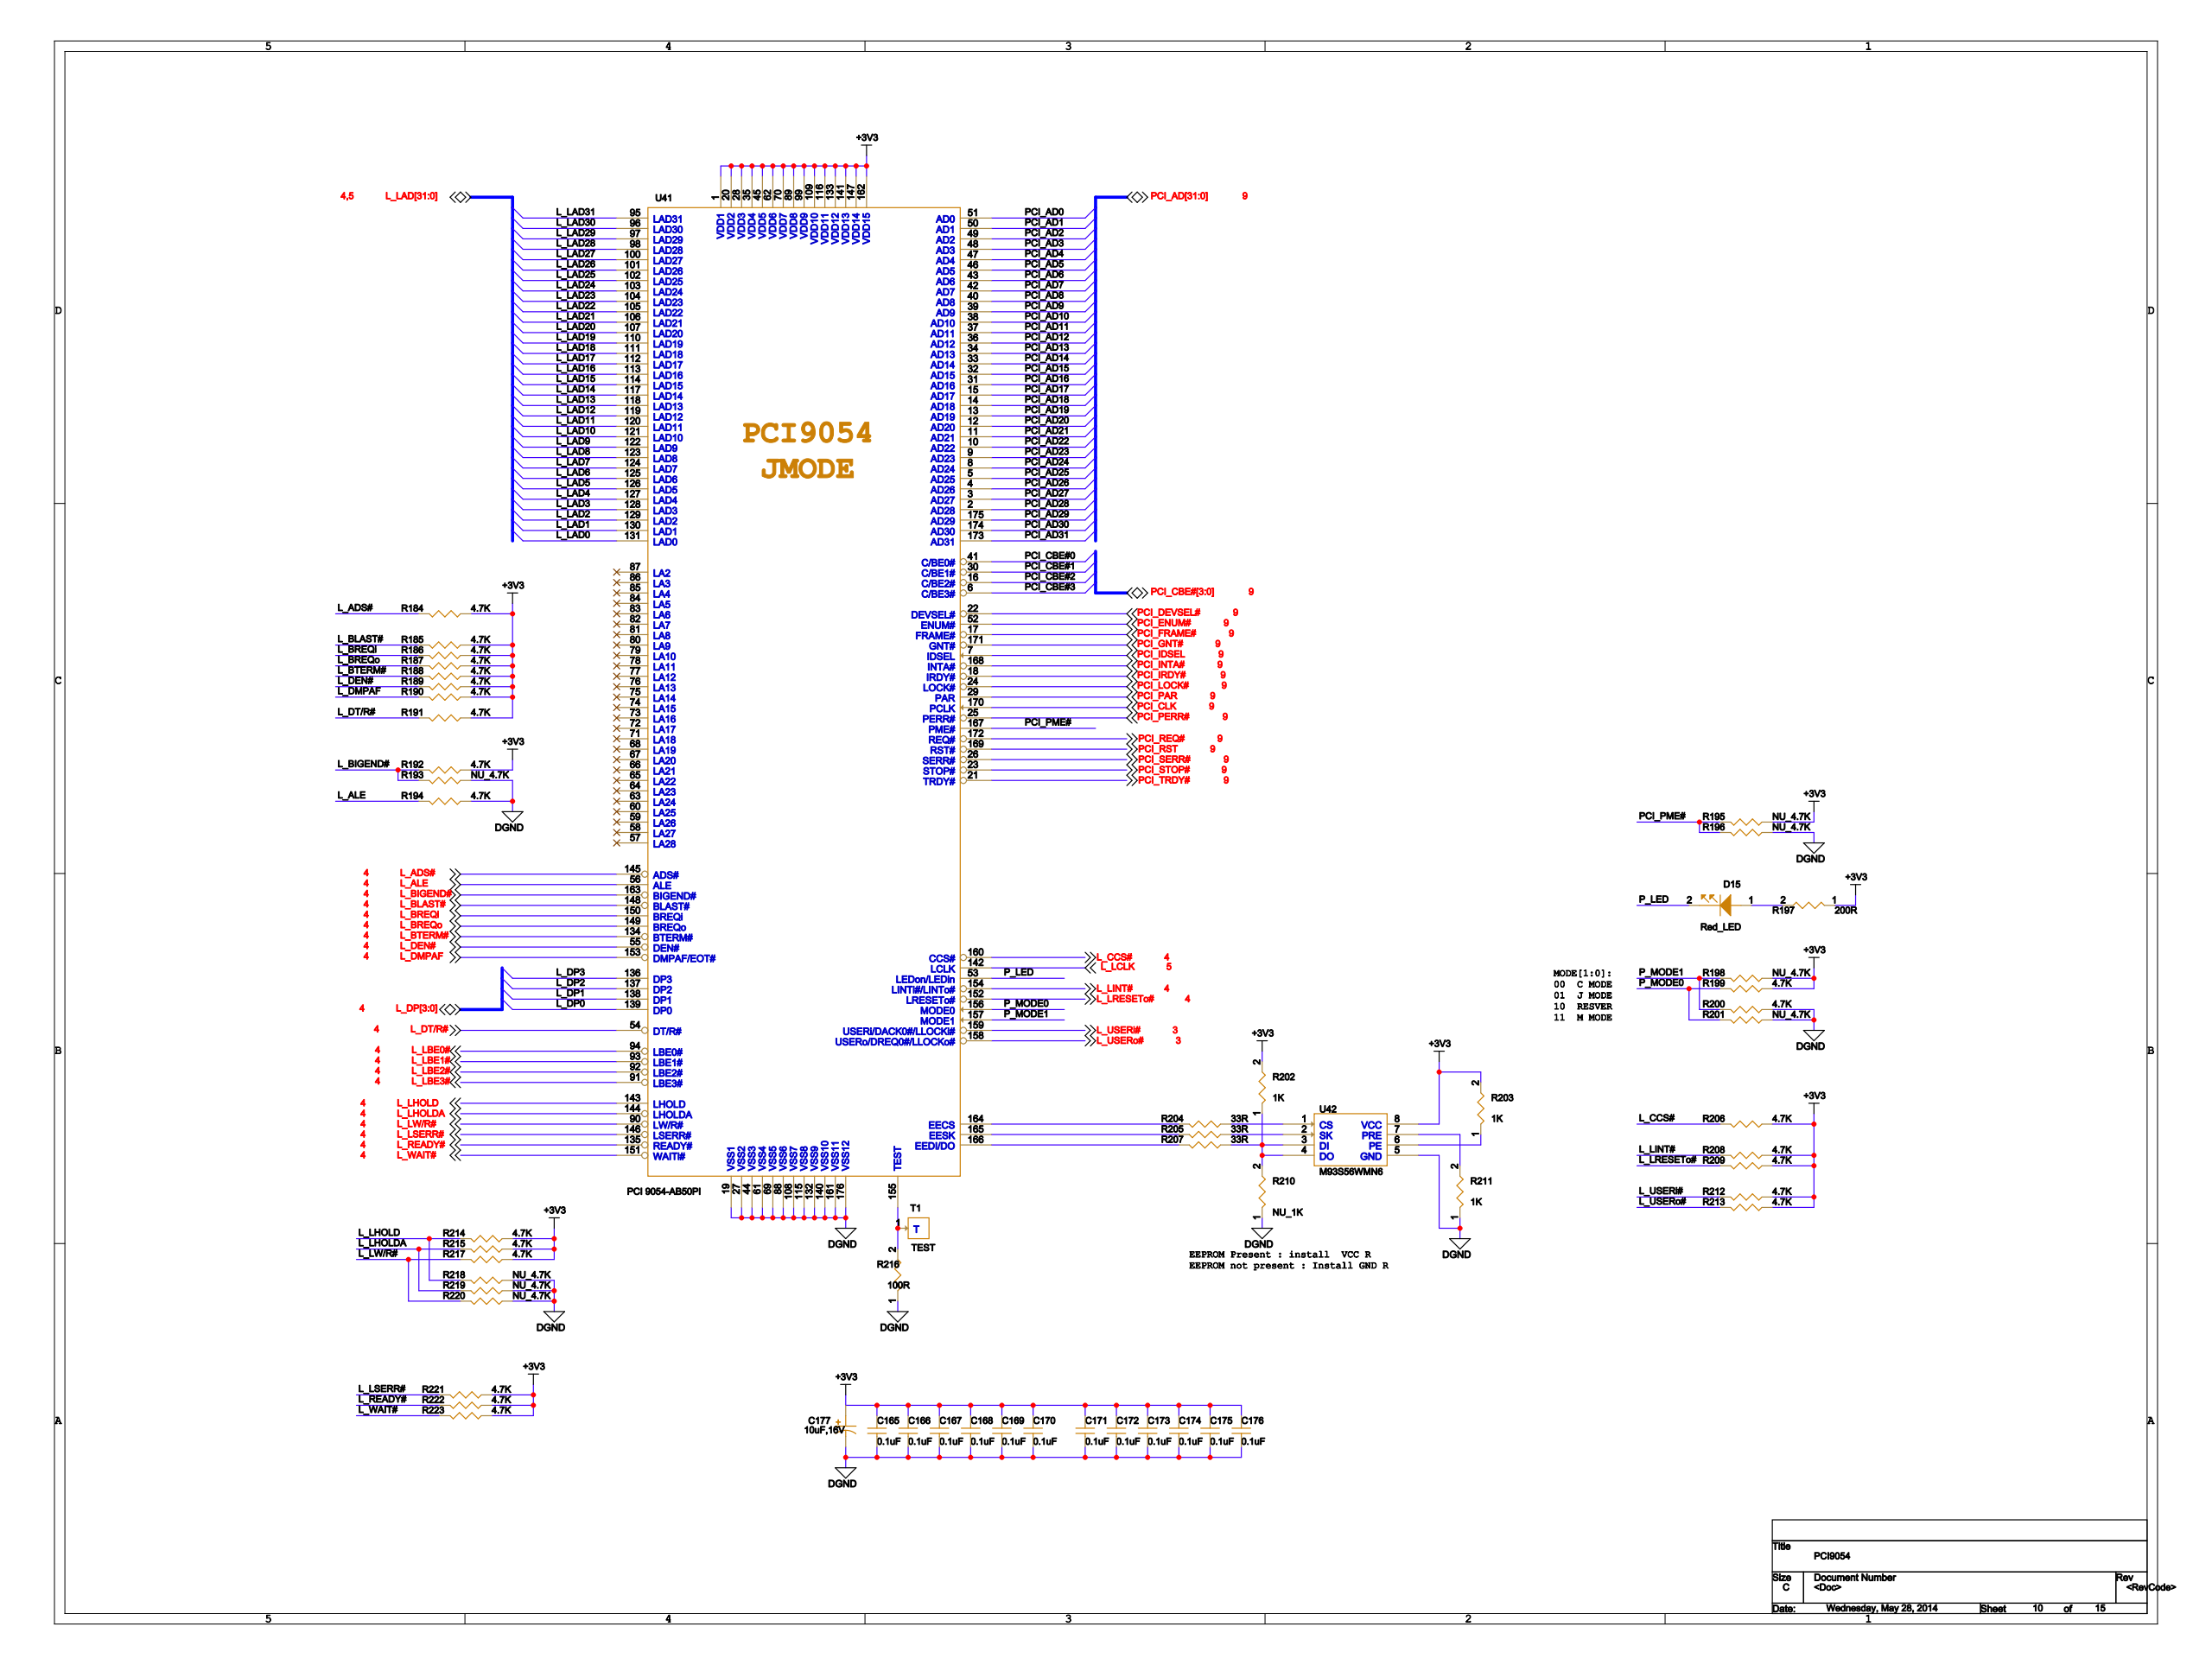Circuit board | Cadence Allegro | 669 parts | 806 nets | one sheet of the schematic
Parts on this sheet (reference | value | footprint):
C165 | 0.1uF | C0402
C166 | 0.1uF | C0402
C167 | 0.1uF | C0402
C168 | 0.1uF | C0402
C169 | 0.1uF | C0402
C170 | 0.1uF | C0402
C171 | 0.1uF | C0402
C172 | 0.1uF | C0402
C173 | 0.1uF | C0402
C174 | 0.1uF | C0402
C175 | 0.1uF | C0402
C176 | 0.1uF | C0402
C177 | 10uF,16V | CP3216
D15 | Red_LED | D0805
R184 | 4.7K | R0603
R185 | 4.7K | R0603
R186 | 4.7K | R0603
R187 | 4.7K | R0603
R188 | 4.7K | R0603
R189 | 4.7K | R0603
R190 | 4.7K | R0603
R191 | 4.7K | R0603
R192 | 4.7K | R0603
R193 | NU_4.7K | R0603
R194 | 4.7K | R0603
R195 | NU_4.7K | R0603
R196 | NU_4.7K | R0603
R197 | 200R | R0603
R198 | NU_4.7K | R0603
R199 | 4.7K | R0603
R200 | 4.7K | R0603
R201 | NU_4.7K | R0603
R202 | 1K | R0603
R203 | 1K | R0603
R204 | 33R | R0603
R205 | 33R | R0603
R206 | 4.7K | R0603
R207 | 33R | R0603
R208 | 4.7K | R0603
R209 | 4.7K | R0603
R210 | NU_1K | R0603
R211 | 1K | R0603
R212 | 4.7K | R0603
R213 | 4.7K | R0603
R214 | 4.7K | R0603
R215 | 4.7K | R0603
R216 | 100R | R0603
R217 | 4.7K | R0603
R218 | NU_4.7K | R0603
R219 | NU_4.7K | R0603
R220 | NU_4.7K | R0603
R221 | 4.7K | R0603
R222 | 4.7K | R0603
R223 | 4.7K | R0603
U41 | PCI 9054-AB50PI | PQFP176
U42 | M93S56WMN6 | SO8
Nets of these parts (net: part-pin ...):
DGND: C165-2 C166-2 C167-2 C168-2 C169-2 C170-2 C171-2 C172-2 C173-2 C174-2 C175-2 C176-2 C177-2 R193-2 R194-2 R196-2 R200-2 R201-2 R210-1 R211-1 R216-1 R218-2 R219-2 R220-2 U42-5 U41-19 U41-27 U41-44 U41-61 U41-69 U41-88 U41-108 U41-115 U41-132 U41-140 U41-161 U41-176
+3V3: C165-1 C166-1 C167-1 C168-1 C169-1 C170-1 C171-1 C172-1 C173-1 C174-1 C175-1 C176-1 C177-1 R184-2 R185-2 R186-2 R187-2 R188-2 R189-2 R190-2 R191-2 R192-2 R195-2 R197-1 R198-2 R199-2 R202-2 R203-2 R206-2 R208-2 R209-2 R212-2 R213-2 R214-2 R215-2 R217-2 R221-2 R222-2 R223-2 U42-8 U41-1 U41-20 U41-28 U41-35 U41-45 U41-62 U41-70 U41-89 U41-99 U41-109 U41-116 U41-133 U41-141 U41-147 U41-162
L_LHOLDA: R215-1 R219-1 U41-144
L_ALE: R194-1 U41-56
L_DT/R#: R191-1 U41-54
L_LAD18: U41-111
L_USERO#: R213-1 U41-158
L_DP3: U41-136
L_READY#: R222-1 U41-135
L_LHOLD: R214-1 R218-1 U41-143
L_DP0: U41-139
L_DP2: U41-137
L_DP1: U41-138
L_BLAST#: R185-1 U41-148
L_LSERR#: R221-1 U41-146
L_LAD5: U41-126
L_ADS#: R184-1 U41-145
L_BREQI: R186-1 U41-150
L_LAD6: U41-125
L_CCS#: R206-1 U41-160
L_LAD4: U41-127
L_BIGEND#: R192-1 R193-1 U41-163
L_BREQO: R187-1 U41-149
L_LRESETO#: R209-1 U41-152
L_WAIT#: R223-1 U41-151
L_LINT#: R208-1 U41-154
L_DMPAF: R190-1 U41-153
L_LAD13: U41-118
L_LAD29: U41-97
L_LAD12: U41-119
L_LAD31: U41-95
L_LAD30: U41-96
L_LAD25: U41-102
L_LAD24: U41-103
L_LAD23: U41-104
L_LAD22: U41-105
L_BTERM#: R188-1 U41-134
L_LAD27: U41-100
L_LAD26: U41-101
L_LW/R#: R217-1 R220-1 U41-90
L_LAD21: U41-106
L_LAD20: U41-107
L_LAD2: U41-129
L_LAD7: U41-124
L_LAD3: U41-128
L_LAD0: U41-131
L_LAD1: U41-130
L_LAD10: U41-121
L_LAD11: U41-120
L_USERI#: R212-1 U41-159
L_LAD19: U41-110
L_LAD17: U41-112
L_LAD15: U41-114
L_LAD14: U41-117
L_LAD16: U41-113
L_LBE2#: U41-92
L_LBE3#: U41-91
L_DEN#: R189-1 U41-55
L_LAD8: U41-123
L_LAD9: U41-122
L_LBE0#: U41-94
L_LBE1#: U41-93
L_LAD28: U41-98
PCI_PME#: R195-1 R196-1 U41-167
P_MODE1: R198-1 R200-1 U41-157
P_MODE0: R199-1 R201-1 U41-156
N47200595: R202-1 R207-2 R210-2 U42-3 U42-4
N47201185: R204-1 U41-164
N47202456: R204-2 U42-1
N47201217: R205-1 U41-165
N47202277: R205-2 U42-2
N47201252: R207-1 U41-166
PCI_ENUM#: U41-52
PCI_FRAME#: U41-17
PCI_IRDY#: U41-18
PCI_TRDY#: U41-21
PCI_DEVSEL#: U41-22
PCI_SERR#: U41-26
PCI_PERR#: U41-25
PCI_LOCK#: U41-24
PCI_PAR: U41-29
PCI_STOP#: U41-23
PCI_RST: U41-169
PCI_IDSEL: U41-7
PCI_CBE#0: U41-41
PCI_INTA#: U41-168
PCI_CBE#1: U41-30
PCI_CBE#2: U41-16
PCI_CBE#3: U41-6
N47201215: D15-1 R197-2
N60830984: R216-2 U41-155
L_LCLK: U41-142
PCI_AD0: U41-51
PCI_AD1: U41-50
PCI_AD2: U41-49
PCI_AD3: U41-48
PCI_AD4: U41-47
PCI_AD5: U41-46
PCI_AD6: U41-43
PCI_AD7: U41-42
PCI_AD8: U41-40
PCI_AD9: U41-39
PCI_AD10: U41-38
PCI_AD11: U41-37
PCI_AD12: U41-36
PCI_AD13: U41-34
PCI_AD14: U41-33
PCI_AD15: U41-32
PCI_AD16: U41-31
PCI_AD17: U41-15
PCI_AD18: U41-14
PCI_AD19: U41-13
PCI_AD20: U41-12
PCI_AD21: U41-11
PCI_AD22: U41-10
PCI_AD23: U41-9
PCI_AD24: U41-8
PCI_AD25: U41-5
PCI_AD26: U41-4
PCI_AD27: U41-3
PCI_AD28: U41-2
PCI_AD29: U41-175
PCI_AD30: U41-174
PCI_AD31: U41-173
P_LED: D15-2 U41-53
PCI_CLK: U41-170
PCI_GNT#: U41-171
PCI_REQ#: U41-172
N47201034: R203-1 U42-6
N47201036: R211-2 U42-7